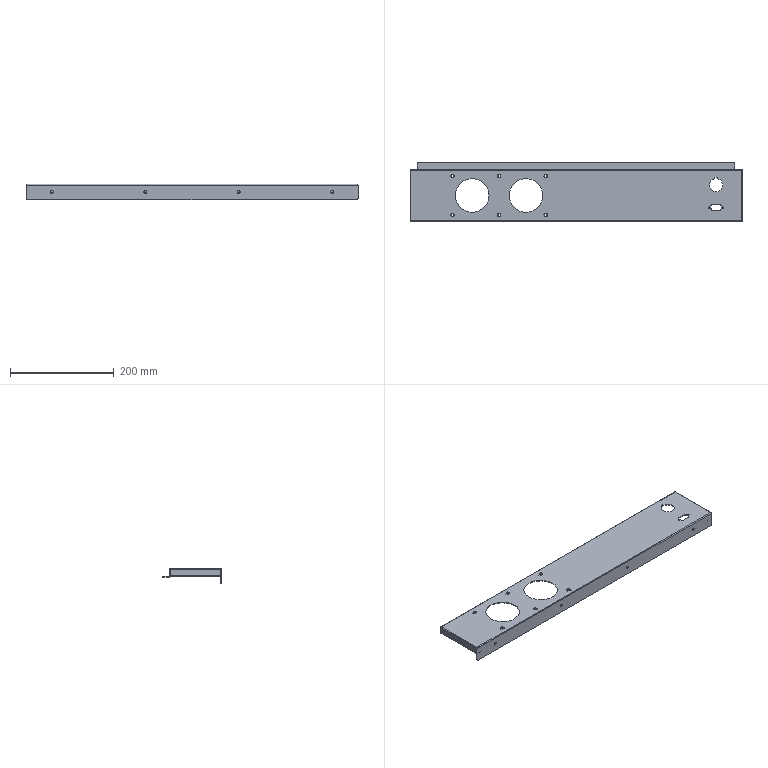Part | STEP file | HESS-408-70-15W-D-4-electrical box bottom plate | 1 solid | 165 faces | box 640 x 113.5 x 30 mm | volume 146678 mm3 | plane 95 | cylinder 70 | commonest cylinder face diameters 5 x19 7 x12 5.5 x8 0.2 x7 3.2 x7 3 x4